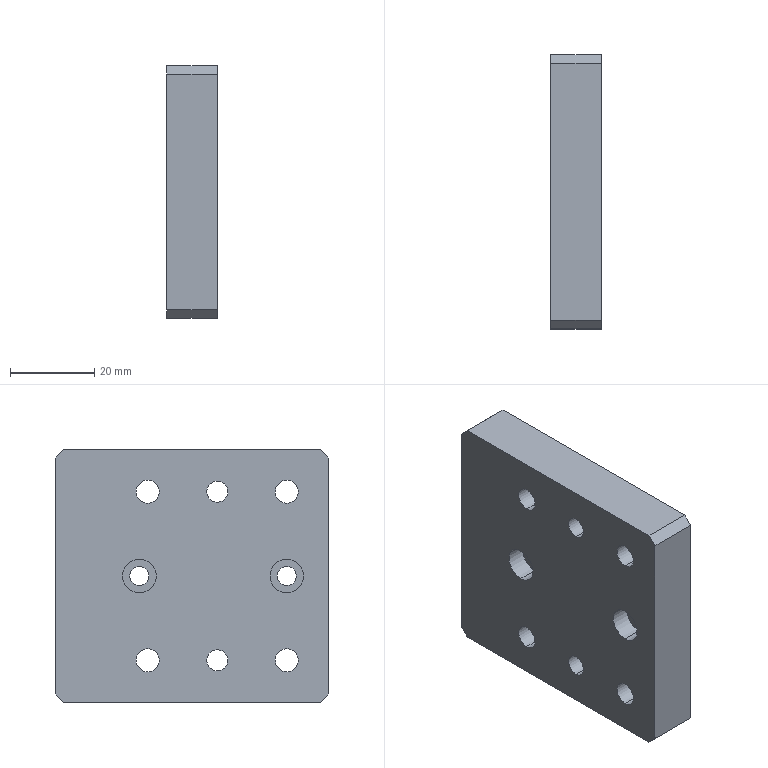Part | SolidWorks | features HoleWzd 3, Chamfer 1, Extrusion 1 | 1 solid | 44 faces | box 12 x 65 x 60 mm | volume 43146 mm3 | cylinder 28 | plane 16 | commonest cylinder face diameters 5.5 x8 10 x8 4.5 x4 5 x4 8 x4
STEP:
#1=CARTESIAN_POINT('',(0.,-6.,-17.5));
#2=VERTEX_POINT('',#1);
#3=CARTESIAN_POINT('',(0.,-6.,-22.5));
#4=VERTEX_POINT('',#3);
#5=CARTESIAN_POINT('',(0.,-6.,-20.));
#6=DIRECTION('',(1.,0.,0.));
#7=DIRECTION('',(0.,0.,-1.));
#8=AXIS2_PLACEMENT_3D('',#5,#6,#7);
#9=CIRCLE('',#8,2.5);
#10=EDGE_CURVE('',#2,#4,#9,.T.);
#11=ORIENTED_EDGE('',*,*,#10,.F.);
#12=CARTESIAN_POINT('',(12.,-6.,-17.5));
#13=VERTEX_POINT('',#12);
#14=CARTESIAN_POINT('',(12.,-6.,-17.5));
#15=DIRECTION('',(1.,0.,0.));
#16=VECTOR('',#15,1000.);
#17=LINE('',#14,#16);
#18=EDGE_CURVE('',#2,#13,#17,.T.);
#19=ORIENTED_EDGE('',*,*,#18,.T.);
#20=CARTESIAN_POINT('',(12.,-6.,-22.5));
#21=VERTEX_POINT('',#20);
#22=CARTESIAN_POINT('',(12.,-6.,-20.));
#23=DIRECTION('',(1.,0.,0.));
#24=DIRECTION('',(0.,0.,-1.));
#25=AXIS2_PLACEMENT_3D('',#22,#23,#24);
#26=CIRCLE('',#25,2.5);
#27=EDGE_CURVE('',#13,#21,#26,.T.);
#28=ORIENTED_EDGE('',*,*,#27,.T.);
#29=CARTESIAN_POINT('',(12.,-6.,-22.5));
#30=DIRECTION('',(1.,0.,0.));
#31=VECTOR('',#30,1000.);
#32=LINE('',#29,#31);
#33=EDGE_CURVE('',#4,#21,#32,.T.);
#34=ORIENTED_EDGE('',*,*,#33,.F.);
#35=EDGE_LOOP('',(#11,#19,#28,#34));
#36=FACE_OUTER_BOUND('',#35,.T.);
#37=CARTESIAN_POINT('',(12.,-6.,-20.));
#38=DIRECTION('',(1.,0.,0.));
#39=DIRECTION('',(0.,0.,-1.));
#40=AXIS2_PLACEMENT_3D('',#37,#38,#39);
#41=CYLINDRICAL_SURFACE('',#40,2.5);
#42=ADVANCED_FACE('',(#36),#41,.F.);
#43=CARTESIAN_POINT('',(0.,-6.,22.5));
#44=VERTEX_POINT('',#43);
#45=CARTESIAN_POINT('',(0.,-6.,17.5));
#46=VERTEX_POINT('',#45);
#47=CARTESIAN_POINT('',(0.,-6.,20.));
#48=DIRECTION('',(1.,0.,0.));
#49=DIRECTION('',(0.,0.,-1.));
#50=AXIS2_PLACEMENT_3D('',#47,#48,#49);
#51=CIRCLE('',#50,2.5);
#52=EDGE_CURVE('',#44,#46,#51,.T.);
#53=ORIENTED_EDGE('',*,*,#52,.F.);
#54=CARTESIAN_POINT('',(12.,-6.,22.5));
#55=VERTEX_POINT('',#54);
#56=CARTESIAN_POINT('',(12.,-6.,22.5));
#57=DIRECTION('',(1.,0.,0.));
#58=VECTOR('',#57,1000.);
#59=LINE('',#56,#58);
#60=EDGE_CURVE('',#44,#55,#59,.T.);
#61=ORIENTED_EDGE('',*,*,#60,.T.);
#62=CARTESIAN_POINT('',(12.,-6.,17.5));
#63=VERTEX_POINT('',#62);
#64=CARTESIAN_POINT('',(12.,-6.,20.));
#65=DIRECTION('',(1.,0.,0.));
#66=DIRECTION('',(0.,0.,-1.));
#67=AXIS2_PLACEMENT_3D('',#64,#65,#66);
#68=CIRCLE('',#67,2.5);
#69=EDGE_CURVE('',#55,#63,#68,.T.);
#70=ORIENTED_EDGE('',*,*,#69,.T.);
#71=CARTESIAN_POINT('',(12.,-6.,17.5));
#72=DIRECTION('',(1.,0.,0.));
#73=VECTOR('',#72,1000.);
#74=LINE('',#71,#73);
#75=EDGE_CURVE('',#46,#63,#74,.T.);
#76=ORIENTED_EDGE('',*,*,#75,.F.);
#77=EDGE_LOOP('',(#53,#61,#70,#76));
#78=FACE_OUTER_BOUND('',#77,.T.);
#79=CARTESIAN_POINT('',(12.,-6.,20.));
#80=DIRECTION('',(1.,0.,0.));
#81=DIRECTION('',(0.,0.,-1.));
#82=AXIS2_PLACEMENT_3D('',#79,#80,#81);
#83=CYLINDRICAL_SURFACE('',#82,2.5);
#84=ADVANCED_FACE('',(#78),#83,.F.);
#85=CARTESIAN_POINT('',(6.3,10.5,25.));
#86=VERTEX_POINT('',#85);
#87=CARTESIAN_POINT('',(6.3,10.5,15.));
#88=VERTEX_POINT('',#87);
#89=CARTESIAN_POINT('',(6.3,10.5,20.));
#90=DIRECTION('',(1.,0.,0.));
#91=DIRECTION('',(0.,0.,-1.));
#92=AXIS2_PLACEMENT_3D('',#89,#90,#91);
#93=CIRCLE('',#92,5.);
#94=EDGE_CURVE('',#86,#88,#93,.T.);
#95=ORIENTED_EDGE('',*,*,#94,.F.);
#96=CARTESIAN_POINT('',(12.,10.5,25.));
#97=VERTEX_POINT('',#96);
#98=CARTESIAN_POINT('',(12.,10.5,25.));
#99=DIRECTION('',(1.,0.,0.));
#100=VECTOR('',#99,1000.);
#101=LINE('',#98,#100);
#102=EDGE_CURVE('',#86,#97,#101,.T.);
#103=ORIENTED_EDGE('',*,*,#102,.T.);
#104=CARTESIAN_POINT('',(12.,10.5,15.));
#105=VERTEX_POINT('',#104);
#106=CARTESIAN_POINT('',(12.,10.5,20.));
#107=DIRECTION('',(1.,0.,0.));
#108=DIRECTION('',(0.,0.,-1.));
#109=AXIS2_PLACEMENT_3D('',#106,#107,#108);
#110=CIRCLE('',#109,5.);
#111=EDGE_CURVE('',#97,#105,#110,.T.);
#112=ORIENTED_EDGE('',*,*,#111,.T.);
#113=CARTESIAN_POINT('',(12.,10.5,15.));
#114=DIRECTION('',(1.,0.,0.));
#115=VECTOR('',#114,1000.);
#116=LINE('',#113,#115);
#117=EDGE_CURVE('',#88,#105,#116,.T.);
#118=ORIENTED_EDGE('',*,*,#117,.F.);
#119=EDGE_LOOP('',(#95,#103,#112,#118));
#120=FACE_OUTER_BOUND('',#119,.T.);
#121=CARTESIAN_POINT('',(12.,10.5,20.));
#122=DIRECTION('',(1.,0.,0.));
#123=DIRECTION('',(0.,0.,-1.));
#124=AXIS2_PLACEMENT_3D('',#121,#122,#123);
#125=CYLINDRICAL_SURFACE('',#124,5.);
#126=ADVANCED_FACE('',(#120),#125,.F.);
#127=CARTESIAN_POINT('',(0.,10.5,22.75));
#128=VERTEX_POINT('',#127);
#129=CARTESIAN_POINT('',(0.,10.5,17.25));
#130=VERTEX_POINT('',#129);
#131=CARTESIAN_POINT('',(0.,10.5,20.));
#132=DIRECTION('',(1.,0.,0.));
#133=DIRECTION('',(0.,0.,-1.));
#134=AXIS2_PLACEMENT_3D('',#131,#132,#133);
#135=CIRCLE('',#134,2.75);
#136=EDGE_CURVE('',#128,#130,#135,.T.);
#137=ORIENTED_EDGE('',*,*,#136,.F.);
#138=CARTESIAN_POINT('',(6.3,10.5,22.75));
#139=VERTEX_POINT('',#138);
#140=CARTESIAN_POINT('',(12.,10.5,22.75));
#141=DIRECTION('',(1.,0.,0.));
#142=VECTOR('',#141,1000.);
#143=LINE('',#140,#142);
#144=EDGE_CURVE('',#128,#139,#143,.T.);
#145=ORIENTED_EDGE('',*,*,#144,.T.);
#146=CARTESIAN_POINT('',(6.3,10.5,17.25));
#147=VERTEX_POINT('',#146);
#148=CARTESIAN_POINT('',(6.3,10.5,20.));
#149=DIRECTION('',(1.,0.,0.));
#150=DIRECTION('',(0.,0.,-1.));
#151=AXIS2_PLACEMENT_3D('',#148,#149,#150);
#152=CIRCLE('',#151,2.75);
#153=EDGE_CURVE('',#139,#147,#152,.T.);
#154=ORIENTED_EDGE('',*,*,#153,.T.);
#155=CARTESIAN_POINT('',(12.,10.5,17.25));
#156=DIRECTION('',(1.,0.,0.));
#157=VECTOR('',#156,1000.);
#158=LINE('',#155,#157);
#159=EDGE_CURVE('',#130,#147,#158,.T.);
#160=ORIENTED_EDGE('',*,*,#159,.F.);
#161=EDGE_LOOP('',(#137,#145,#154,#160));
#162=FACE_OUTER_BOUND('',#161,.T.);
#163=CARTESIAN_POINT('',(12.,10.5,20.));
#164=DIRECTION('',(1.,0.,0.));
#165=DIRECTION('',(0.,0.,-1.));
#166=AXIS2_PLACEMENT_3D('',#163,#164,#165);
#167=CYLINDRICAL_SURFACE('',#166,2.75);
#168=ADVANCED_FACE('',(#162),#167,.F.);
#169=CARTESIAN_POINT('',(6.3,-22.5,25.));
#170=VERTEX_POINT('',#169);
#171=CARTESIAN_POINT('',(6.3,-22.5,15.));
#172=VERTEX_POINT('',#171);
#173=CARTESIAN_POINT('',(6.3,-22.5,20.));
#174=DIRECTION('',(1.,0.,0.));
#175=DIRECTION('',(0.,0.,-1.));
#176=AXIS2_PLACEMENT_3D('',#173,#174,#175);
#177=CIRCLE('',#176,5.);
#178=EDGE_CURVE('',#170,#172,#177,.T.);
#179=ORIENTED_EDGE('',*,*,#178,.F.);
#180=CARTESIAN_POINT('',(12.,-22.5,25.));
#181=VERTEX_POINT('',#180);
#182=CARTESIAN_POINT('',(12.,-22.5,25.));
#183=DIRECTION('',(1.,0.,0.));
#184=VECTOR('',#183,1000.);
#185=LINE('',#182,#184);
#186=EDGE_CURVE('',#170,#181,#185,.T.);
#187=ORIENTED_EDGE('',*,*,#186,.T.);
#188=CARTESIAN_POINT('',(12.,-22.5,15.));
#189=VERTEX_POINT('',#188);
#190=CARTESIAN_POINT('',(12.,-22.5,20.));
#191=DIRECTION('',(1.,0.,0.));
#192=DIRECTION('',(0.,0.,-1.));
#193=AXIS2_PLACEMENT_3D('',#190,#191,#192);
#194=CIRCLE('',#193,5.);
#195=EDGE_CURVE('',#181,#189,#194,.T.);
#196=ORIENTED_EDGE('',*,*,#195,.T.);
#197=CARTESIAN_POINT('',(12.,-22.5,15.));
#198=DIRECTION('',(1.,0.,0.));
#199=VECTOR('',#198,1000.);
#200=LINE('',#197,#199);
#201=EDGE_CURVE('',#172,#189,#200,.T.);
#202=ORIENTED_EDGE('',*,*,#201,.F.);
#203=EDGE_LOOP('',(#179,#187,#196,#202));
#204=FACE_OUTER_BOUND('',#203,.T.);
#205=CARTESIAN_POINT('',(12.,-22.5,20.));
#206=DIRECTION('',(1.,0.,0.));
#207=DIRECTION('',(0.,0.,-1.));
#208=AXIS2_PLACEMENT_3D('',#205,#206,#207);
#209=CYLINDRICAL_SURFACE('',#208,5.);
#210=ADVANCED_FACE('',(#204),#209,.F.);
#211=CARTESIAN_POINT('',(0.,-22.5,22.75));
#212=VERTEX_POINT('',#211);
#213=CARTESIAN_POINT('',(0.,-22.5,17.25));
#214=VERTEX_POINT('',#213);
#215=CARTESIAN_POINT('',(0.,-22.5,20.));
#216=DIRECTION('',(1.,0.,0.));
#217=DIRECTION('',(0.,0.,-1.));
#218=AXIS2_PLACEMENT_3D('',#215,#216,#217);
#219=CIRCLE('',#218,2.75);
#220=EDGE_CURVE('',#212,#214,#219,.T.);
#221=ORIENTED_EDGE('',*,*,#220,.F.);
#222=CARTESIAN_POINT('',(6.3,-22.5,22.75));
#223=VERTEX_POINT('',#222);
#224=CARTESIAN_POINT('',(12.,-22.5,22.75));
#225=DIRECTION('',(1.,0.,0.));
#226=VECTOR('',#225,1000.);
#227=LINE('',#224,#226);
#228=EDGE_CURVE('',#212,#223,#227,.T.);
#229=ORIENTED_EDGE('',*,*,#228,.T.);
#230=CARTESIAN_POINT('',(6.3,-22.5,17.25));
#231=VERTEX_POINT('',#230);
#232=CARTESIAN_POINT('',(6.3,-22.5,20.));
#233=DIRECTION('',(1.,0.,0.));
#234=DIRECTION('',(0.,0.,-1.));
#235=AXIS2_PLACEMENT_3D('',#232,#233,#234);
#236=CIRCLE('',#235,2.75);
#237=EDGE_CURVE('',#223,#231,#236,.T.);
#238=ORIENTED_EDGE('',*,*,#237,.T.);
#239=CARTESIAN_POINT('',(12.,-22.5,17.25));
#240=DIRECTION('',(1.,0.,0.));
#241=VECTOR('',#240,1000.);
#242=LINE('',#239,#241);
#243=EDGE_CURVE('',#214,#231,#242,.T.);
#244=ORIENTED_EDGE('',*,*,#243,.F.);
#245=EDGE_LOOP('',(#221,#229,#238,#244));
#246=FACE_OUTER_BOUND('',#245,.T.);
#247=CARTESIAN_POINT('',(12.,-22.5,20.));
#248=DIRECTION('',(1.,0.,0.));
#249=DIRECTION('',(0.,0.,-1.));
#250=AXIS2_PLACEMENT_3D('',#247,#248,#249);
#251=CYLINDRICAL_SURFACE('',#250,2.75);
#252=ADVANCED_FACE('',(#246),#251,.F.);
#253=CARTESIAN_POINT('',(6.3,-22.5,-15.));
#254=VERTEX_POINT('',#253);
#255=CARTESIAN_POINT('',(6.3,-22.5,-25.));
#256=VERTEX_POINT('',#255);
#257=CARTESIAN_POINT('',(6.3,-22.5,-20.));
#258=DIRECTION('',(1.,0.,0.));
#259=DIRECTION('',(0.,0.,-1.));
#260=AXIS2_PLACEMENT_3D('',#257,#258,#259);
#261=CIRCLE('',#260,5.);
#262=EDGE_CURVE('',#254,#256,#261,.T.);
#263=ORIENTED_EDGE('',*,*,#262,.F.);
#264=CARTESIAN_POINT('',(12.,-22.5,-15.));
#265=VERTEX_POINT('',#264);
#266=CARTESIAN_POINT('',(12.,-22.5,-15.));
#267=DIRECTION('',(1.,0.,0.));
#268=VECTOR('',#267,1000.);
#269=LINE('',#266,#268);
#270=EDGE_CURVE('',#254,#265,#269,.T.);
#271=ORIENTED_EDGE('',*,*,#270,.T.);
#272=CARTESIAN_POINT('',(12.,-22.5,-25.));
#273=VERTEX_POINT('',#272);
#274=CARTESIAN_POINT('',(12.,-22.5,-20.));
#275=DIRECTION('',(1.,0.,0.));
#276=DIRECTION('',(0.,0.,-1.));
#277=AXIS2_PLACEMENT_3D('',#274,#275,#276);
#278=CIRCLE('',#277,5.);
#279=EDGE_CURVE('',#265,#273,#278,.T.);
#280=ORIENTED_EDGE('',*,*,#279,.T.);
#281=CARTESIAN_POINT('',(12.,-22.5,-25.));
#282=DIRECTION('',(1.,0.,0.));
#283=VECTOR('',#282,1000.);
#284=LINE('',#281,#283);
#285=EDGE_CURVE('',#256,#273,#284,.T.);
#286=ORIENTED_EDGE('',*,*,#285,.F.);
#287=EDGE_LOOP('',(#263,#271,#280,#286));
#288=FACE_OUTER_BOUND('',#287,.T.);
#289=CARTESIAN_POINT('',(12.,-22.5,-20.));
#290=DIRECTION('',(1.,0.,0.));
#291=DIRECTION('',(0.,0.,-1.));
#292=AXIS2_PLACEMENT_3D('',#289,#290,#291);
#293=CYLINDRICAL_SURFACE('',#292,5.);
#294=ADVANCED_FACE('',(#288),#293,.F.);
#295=CARTESIAN_POINT('',(0.,-22.5,-17.25));
#296=VERTEX_POINT('',#295);
#297=CARTESIAN_POINT('',(0.,-22.5,-22.75));
#298=VERTEX_POINT('',#297);
#299=CARTESIAN_POINT('',(0.,-22.5,-20.));
#300=DIRECTION('',(1.,0.,0.));
#301=DIRECTION('',(0.,0.,-1.));
#302=AXIS2_PLACEMENT_3D('',#299,#300,#301);
#303=CIRCLE('',#302,2.75);
#304=EDGE_CURVE('',#296,#298,#303,.T.);
#305=ORIENTED_EDGE('',*,*,#304,.F.);
#306=CARTESIAN_POINT('',(6.3,-22.5,-17.25));
#307=VERTEX_POINT('',#306);
#308=CARTESIAN_POINT('',(12.,-22.5,-17.25));
#309=DIRECTION('',(1.,0.,0.));
#310=VECTOR('',#309,1000.);
#311=LINE('',#308,#310);
#312=EDGE_CURVE('',#296,#307,#311,.T.);
#313=ORIENTED_EDGE('',*,*,#312,.T.);
#314=CARTESIAN_POINT('',(6.3,-22.5,-22.75));
#315=VERTEX_POINT('',#314);
#316=CARTESIAN_POINT('',(6.3,-22.5,-20.));
#317=DIRECTION('',(1.,0.,0.));
#318=DIRECTION('',(0.,0.,-1.));
#319=AXIS2_PLACEMENT_3D('',#316,#317,#318);
#320=CIRCLE('',#319,2.75);
#321=EDGE_CURVE('',#307,#315,#320,.T.);
#322=ORIENTED_EDGE('',*,*,#321,.T.);
#323=CARTESIAN_POINT('',(12.,-22.5,-22.75));
#324=DIRECTION('',(1.,0.,0.));
#325=VECTOR('',#324,1000.);
#326=LINE('',#323,#325);
#327=EDGE_CURVE('',#298,#315,#326,.T.);
#328=ORIENTED_EDGE('',*,*,#327,.F.);
#329=EDGE_LOOP('',(#305,#313,#322,#328));
#330=FACE_OUTER_BOUND('',#329,.T.);
#331=CARTESIAN_POINT('',(12.,-22.5,-20.));
#332=DIRECTION('',(1.,0.,0.));
#333=DIRECTION('',(0.,0.,-1.));
#334=AXIS2_PLACEMENT_3D('',#331,#332,#333);
#335=CYLINDRICAL_SURFACE('',#334,2.75);
#336=ADVANCED_FACE('',(#330),#335,.F.);
#337=CARTESIAN_POINT('',(6.3,10.5,-15.));
#338=VERTEX_POINT('',#337);
#339=CARTESIAN_POINT('',(6.3,10.5,-25.));
#340=VERTEX_POINT('',#339);
#341=CARTESIAN_POINT('',(6.3,10.5,-20.));
#342=DIRECTION('',(1.,0.,0.));
#343=DIRECTION('',(0.,0.,-1.));
#344=AXIS2_PLACEMENT_3D('',#341,#342,#343);
#345=CIRCLE('',#344,5.);
#346=EDGE_CURVE('',#338,#340,#345,.T.);
#347=ORIENTED_EDGE('',*,*,#346,.F.);
#348=CARTESIAN_POINT('',(12.,10.5,-15.));
#349=VERTEX_POINT('',#348);
#350=CARTESIAN_POINT('',(12.,10.5,-15.));
#351=DIRECTION('',(1.,0.,0.));
#352=VECTOR('',#351,1000.);
#353=LINE('',#350,#352);
#354=EDGE_CURVE('',#338,#349,#353,.T.);
#355=ORIENTED_EDGE('',*,*,#354,.T.);
#356=CARTESIAN_POINT('',(12.,10.5,-25.));
#357=VERTEX_POINT('',#356);
#358=CARTESIAN_POINT('',(12.,10.5,-20.));
#359=DIRECTION('',(1.,0.,0.));
#360=DIRECTION('',(0.,0.,-1.));
#361=AXIS2_PLACEMENT_3D('',#358,#359,#360);
#362=CIRCLE('',#361,5.);
#363=EDGE_CURVE('',#349,#357,#362,.T.);
#364=ORIENTED_EDGE('',*,*,#363,.T.);
#365=CARTESIAN_POINT('',(12.,10.5,-25.));
#366=DIRECTION('',(1.,0.,0.));
#367=VECTOR('',#366,1000.);
#368=LINE('',#365,#367);
#369=EDGE_CURVE('',#340,#357,#368,.T.);
#370=ORIENTED_EDGE('',*,*,#369,.F.);
#371=EDGE_LOOP('',(#347,#355,#364,#370));
#372=FACE_OUTER_BOUND('',#371,.T.);
#373=CARTESIAN_POINT('',(12.,10.5,-20.));
#374=DIRECTION('',(1.,0.,0.));
#375=DIRECTION('',(0.,0.,-1.));
#376=AXIS2_PLACEMENT_3D('',#373,#374,#375);
#377=CYLINDRICAL_SURFACE('',#376,5.);
#378=ADVANCED_FACE('',(#372),#377,.F.);
#379=CARTESIAN_POINT('',(0.,10.5,-17.25));
#380=VERTEX_POINT('',#379);
#381=CARTESIAN_POINT('',(0.,10.5,-22.75));
#382=VERTEX_POINT('',#381);
#383=CARTESIAN_POINT('',(0.,10.5,-20.));
#384=DIRECTION('',(1.,0.,0.));
#385=DIRECTION('',(0.,0.,-1.));
#386=AXIS2_PLACEMENT_3D('',#383,#384,#385);
#387=CIRCLE('',#386,2.75);
#388=EDGE_CURVE('',#380,#382,#387,.T.);
#389=ORIENTED_EDGE('',*,*,#388,.F.);
#390=CARTESIAN_POINT('',(6.3,10.5,-17.25));
#391=VERTEX_POINT('',#390);
#392=CARTESIAN_POINT('',(12.,10.5,-17.25));
#393=DIRECTION('',(1.,0.,0.));
#394=VECTOR('',#393,1000.);
#395=LINE('',#392,#394);
#396=EDGE_CURVE('',#380,#391,#395,.T.);
#397=ORIENTED_EDGE('',*,*,#396,.T.);
#398=CARTESIAN_POINT('',(6.3,10.5,-22.75));
#399=VERTEX_POINT('',#398);
#400=CARTESIAN_POINT('',(6.3,10.5,-20.));
#401=DIRECTION('',(1.,0.,0.));
#402=DIRECTION('',(0.,0.,-1.));
#403=AXIS2_PLACEMENT_3D('',#400,#401,#402);
#404=CIRCLE('',#403,2.75);
#405=EDGE_CURVE('',#391,#399,#404,.T.);
#406=ORIENTED_EDGE('',*,*,#405,.T.);
#407=CARTESIAN_POINT('',(12.,10.5,-22.75));
#408=DIRECTION('',(1.,0.,0.));
#409=VECTOR('',#408,1000.);
#410=LINE('',#407,#409);
#411=EDGE_CURVE('',#382,#399,#410,.T.);
#412=ORIENTED_EDGE('',*,*,#411,.F.);
#413=EDGE_LOOP('',(#389,#397,#406,#412));
#414=FACE_OUTER_BOUND('',#413,.T.);
#415=CARTESIAN_POINT('',(12.,10.5,-20.));
#416=DIRECTION('',(1.,0.,0.));
#417=DIRECTION('',(0.,0.,-1.));
#418=AXIS2_PLACEMENT_3D('',#415,#416,#417);
#419=CYLINDRICAL_SURFACE('',#418,2.75);
#420=ADVANCED_FACE('',(#414),#419,.F.);
#421=CARTESIAN_POINT('',(4.6,12.5,-4.));
#422=VERTEX_POINT('',#421);
#423=CARTESIAN_POINT('',(4.6,12.5,4.));
#424=VERTEX_POINT('',#423);
#425=CARTESIAN_POINT('',(4.6,12.5,0.));
#426=DIRECTION('',(-1.,0.,0.));
#427=DIRECTION('',(0.,0.,1.));
#428=AXIS2_PLACEMENT_3D('',#425,#426,#427);
#429=CIRCLE('',#428,4.);
#430=EDGE_CURVE('',#422,#424,#429,.T.);
#431=ORIENTED_EDGE('',*,*,#430,.F.);
#432=CARTESIAN_POINT('',(0.,12.5,-4.));
#433=VERTEX_POINT('',#432);
#434=CARTESIAN_POINT('',(0.,12.5,-4.));
#435=DIRECTION('',(-1.,0.,0.));
#436=VECTOR('',#435,1000.);
#437=LINE('',#434,#436);
#438=EDGE_CURVE('',#422,#433,#437,.T.);
#439=ORIENTED_EDGE('',*,*,#438,.T.);
#440=CARTESIAN_POINT('',(0.,12.5,4.));
#441=VERTEX_POINT('',#440);
#442=CARTESIAN_POINT('',(0.,12.5,0.));
#443=DIRECTION('',(-1.,0.,0.));
#444=DIRECTION('',(0.,0.,1.));
#445=AXIS2_PLACEMENT_3D('',#442,#443,#444);
#446=CIRCLE('',#445,4.);
#447=EDGE_CURVE('',#433,#441,#446,.T.);
#448=ORIENTED_EDGE('',*,*,#447,.T.);
#449=CARTESIAN_POINT('',(0.,12.5,4.));
#450=DIRECTION('',(-1.,0.,0.));
#451=VECTOR('',#450,1000.);
#452=LINE('',#449,#451);
#453=EDGE_CURVE('',#424,#441,#452,.T.);
#454=ORIENTED_EDGE('',*,*,#453,.F.);
#455=EDGE_LOOP('',(#431,#439,#448,#454));
#456=FACE_OUTER_BOUND('',#455,.T.);
#457=CARTESIAN_POINT('',(0.,12.5,0.));
#458=DIRECTION('',(-1.,0.,0.));
#459=DIRECTION('',(0.,0.,1.));
#460=AXIS2_PLACEMENT_3D('',#457,#458,#459);
#461=CYLINDRICAL_SURFACE('',#460,4.);
#462=ADVANCED_FACE('',(#456),#461,.F.);
#463=CARTESIAN_POINT('',(12.,12.5,-2.25));
#464=VERTEX_POINT('',#463);
#465=CARTESIAN_POINT('',(12.,12.5,2.25));
#466=VERTEX_POINT('',#465);
#467=CARTESIAN_POINT('',(12.,12.5,0.));
#468=DIRECTION('',(-1.,0.,0.));
#469=DIRECTION('',(0.,0.,1.));
#470=AXIS2_PLACEMENT_3D('',#467,#468,#469);
#471=CIRCLE('',#470,2.25);
#472=EDGE_CURVE('',#464,#466,#471,.T.);
#473=ORIENTED_EDGE('',*,*,#472,.F.);
#474=CARTESIAN_POINT('',(4.6,12.5,-2.25));
#475=VERTEX_POINT('',#474);
#476=CARTESIAN_POINT('',(0.,12.5,-2.25));
#477=DIRECTION('',(-1.,0.,0.));
#478=VECTOR('',#477,1000.);
#479=LINE('',#476,#478);
#480=EDGE_CURVE('',#464,#475,#479,.T.);
#481=ORIENTED_EDGE('',*,*,#480,.T.);
#482=CARTESIAN_POINT('',(4.6,12.5,2.25));
#483=VERTEX_POINT('',#482);
#484=CARTESIAN_POINT('',(4.6,12.5,0.));
#485=DIRECTION('',(-1.,0.,0.));
#486=DIRECTION('',(0.,0.,1.));
#487=AXIS2_PLACEMENT_3D('',#484,#485,#486);
#488=CIRCLE('',#487,2.25);
#489=EDGE_CURVE('',#475,#483,#488,.T.);
#490=ORIENTED_EDGE('',*,*,#489,.T.);
#491=CARTESIAN_POINT('',(0.,12.5,2.25));
#492=DIRECTION('',(-1.,0.,0.));
#493=VECTOR('',#492,1000.);
#494=LINE('',#491,#493);
#495=EDGE_CURVE('',#466,#483,#494,.T.);
#496=ORIENTED_EDGE('',*,*,#495,.F.);
#497=EDGE_LOOP('',(#473,#481,#490,#496));
#498=FACE_OUTER_BOUND('',#497,.T.);
#499=CARTESIAN_POINT('',(0.,12.5,0.));
#500=DIRECTION('',(-1.,0.,0.));
#501=DIRECTION('',(0.,0.,1.));
#502=AXIS2_PLACEMENT_3D('',#499,#500,#501);
#503=CYLINDRICAL_SURFACE('',#502,2.25);
#504=ADVANCED_FACE('',(#498),#503,.F.);
#505=CARTESIAN_POINT('',(4.6,-22.5,-4.));
#506=VERTEX_POINT('',#505);
#507=CARTESIAN_POINT('',(4.6,-22.5,4.));
#508=VERTEX_POINT('',#507);
#509=CARTESIAN_POINT('',(4.6,-22.5,0.));
#510=DIRECTION('',(-1.,0.,0.));
#511=DIRECTION('',(0.,0.,1.));
#512=AXIS2_PLACEMENT_3D('',#509,#510,#511);
#513=CIRCLE('',#512,4.);
#514=EDGE_CURVE('',#506,#508,#513,.T.);
#515=ORIENTED_EDGE('',*,*,#514,.F.);
#516=CARTESIAN_POINT('',(0.,-22.5,-4.));
#517=VERTEX_POINT('',#516);
#518=CARTESIAN_POINT('',(0.,-22.5,-4.));
#519=DIRECTION('',(-1.,0.,0.));
#520=VECTOR('',#519,1000.);
#521=LINE('',#518,#520);
#522=EDGE_CURVE('',#506,#517,#521,.T.);
#523=ORIENTED_EDGE('',*,*,#522,.T.);
#524=CARTESIAN_POINT('',(0.,-22.5,4.));
#525=VERTEX_POINT('',#524);
#526=CARTESIAN_POINT('',(0.,-22.5,0.));
#527=DIRECTION('',(-1.,0.,0.));
#528=DIRECTION('',(0.,0.,1.));
#529=AXIS2_PLACEMENT_3D('',#526,#527,#528);
#530=CIRCLE('',#529,4.);
#531=EDGE_CURVE('',#517,#525,#530,.T.);
#532=ORIENTED_EDGE('',*,*,#531,.T.);
#533=CARTESIAN_POINT('',(0.,-22.5,4.));
#534=DIRECTION('',(-1.,0.,0.));
#535=VECTOR('',#534,1000.);
#536=LINE('',#533,#535);
#537=EDGE_CURVE('',#508,#525,#536,.T.);
#538=ORIENTED_EDGE('',*,*,#537,.F.);
#539=EDGE_LOOP('',(#515,#523,#532,#538));
#540=FACE_OUTER_BOUND('',#539,.T.);
#541=CARTESIAN_POINT('',(0.,-22.5,0.));
#542=DIRECTION('',(-1.,0.,0.));
#543=DIRECTION('',(0.,0.,1.));
#544=AXIS2_PLACEMENT_3D('',#541,#542,#543);
#545=CYLINDRICAL_SURFACE('',#544,4.);
#546=ADVANCED_FACE('',(#540),#545,.F.);
#547=CARTESIAN_POINT('',(12.,-22.5,-2.25));
#548=VERTEX_POINT('',#547);
#549=CARTESIAN_POINT('',(12.,-22.5,2.25));
#550=VERTEX_POINT('',#549);
#551=CARTESIAN_POINT('',(12.,-22.5,0.));
#552=DIRECTION('',(-1.,0.,0.));
#553=DIRECTION('',(0.,0.,1.));
#554=AXIS2_PLACEMENT_3D('',#551,#552,#553);
#555=CIRCLE('',#554,2.25);
#556=EDGE_CURVE('',#548,#550,#555,.T.);
#557=ORIENTED_EDGE('',*,*,#556,.F.);
#558=CARTESIAN_POINT('',(4.6,-22.5,-2.25));
#559=VERTEX_POINT('',#558);
#560=CARTESIAN_POINT('',(0.,-22.5,-2.25));
#561=DIRECTION('',(-1.,0.,0.));
#562=VECTOR('',#561,1000.);
#563=LINE('',#560,#562);
#564=EDGE_CURVE('',#548,#559,#563,.T.);
#565=ORIENTED_EDGE('',*,*,#564,.T.);
#566=CARTESIAN_POINT('',(4.6,-22.5,2.25));
#567=VERTEX_POINT('',#566);
#568=CARTESIAN_POINT('',(4.6,-22.5,0.));
#569=DIRECTION('',(-1.,0.,0.));
#570=DIRECTION('',(0.,0.,1.));
#571=AXIS2_PLACEMENT_3D('',#568,#569,#570);
#572=CIRCLE('',#571,2.25);
#573=EDGE_CURVE('',#559,#567,#572,.T.);
#574=ORIENTED_EDGE('',*,*,#573,.T.);
#575=CARTESIAN_POINT('',(0.,-22.5,2.25));
#576=DIRECTION('',(-1.,0.,0.));
#577=VECTOR('',#576,1000.);
#578=LINE('',#575,#577);
#579=EDGE_CURVE('',#550,#567,#578,.T.);
#580=ORIENTED_EDGE('',*,*,#579,.F.);
#581=EDGE_LOOP('',(#557,#565,#574,#580));
#582=FACE_OUTER_BOUND('',#581,.T.);
#583=CARTESIAN_POINT('',(0.,-22.5,0.));
#584=DIRECTION('',(-1.,0.,0.));
#585=DIRECTION('',(0.,0.,1.));
#586=AXIS2_PLACEMENT_3D('',#583,#584,#585);
#587=CYLINDRICAL_SURFACE('',#586,2.25);
#588=ADVANCED_FACE('',(#582),#587,.F.);
#589=CARTESIAN_POINT('',(12.,-30.5,-30.));
#590=VERTEX_POINT('',#589);
#591=CARTESIAN_POINT('',(12.,30.5,-30.));
#592=VERTEX_POINT('',#591);
#593=CARTESIAN_POINT('',(12.,-32.5,-30.));
#594=DIRECTION('',(0.,1.,0.));
#595=VECTOR('',#594,1000.);
#596=LINE('',#593,#595);
#597=EDGE_CURVE('',#590,#592,#596,.T.);
#598=ORIENTED_EDGE('',*,*,#597,.F.);
#599=CARTESIAN_POINT('',(0.,-30.5,-30.));
#600=VERTEX_POINT('',#599);
#601=CARTESIAN_POINT('',(12.,-30.5,-30.));
#602=DIRECTION('',(-1.,0.,0.));
#603=VECTOR('',#602,1000.);
#604=LINE('',#601,#603);
#605=EDGE_CURVE('',#590,#600,#604,.T.);
#606=ORIENTED_EDGE('',*,*,#605,.T.);
#607=CARTESIAN_POINT('',(0.,30.5,-30.));
#608=VERTEX_POINT('',#607);
#609=CARTESIAN_POINT('',(0.,-32.5,-30.));
#610=DIRECTION('',(0.,1.,0.));
#611=VECTOR('',#610,1000.);
#612=LINE('',#609,#611);
#613=EDGE_CURVE('',#600,#608,#612,.T.);
#614=ORIENTED_EDGE('',*,*,#613,.T.);
#615=CARTESIAN_POINT('',(12.,30.5,-30.));
#616=DIRECTION('',(1.,0.,0.));
#617=VECTOR('',#616,1000.);
#618=LINE('',#615,#617);
#619=EDGE_CURVE('',#608,#592,#618,.T.);
#620=ORIENTED_EDGE('',*,*,#619,.T.);
#621=EDGE_LOOP('',(#598,#606,#614,#620));
#622=FACE_OUTER_BOUND('',#621,.T.);
#623=CARTESIAN_POINT('',(12.,-32.5,-30.));
#624=DIRECTION('',(0.,0.,1.));
#625=DIRECTION('',(1.,0.,0.));
#626=AXIS2_PLACEMENT_3D('',#623,#624,#625);
#627=PLANE('',#626);
#628=ADVANCED_FACE('',(#622),#627,.F.);
#629=CARTESIAN_POINT('',(0.,32.5,-28.));
#630=VERTEX_POINT('',#629);
#631=CARTESIAN_POINT('',(0.,32.5,28.));
#632=VERTEX_POINT('',#631);
#633=CARTESIAN_POINT('',(0.,32.5,30.));
#634=DIRECTION('',(0.,0.,1.));
#635=VECTOR('',#634,1000.);
#636=LINE('',#633,#635);
#637=EDGE_CURVE('',#630,#632,#636,.T.);
#638=ORIENTED_EDGE('',*,*,#637,.T.);
#639=CARTESIAN_POINT('',(12.,32.5,28.));
#640=VERTEX_POINT('',#639);
#641=CARTESIAN_POINT('',(12.,32.5,28.));
#642=DIRECTION('',(1.,0.,0.));
#643=VECTOR('',#642,1000.);
#644=LINE('',#641,#643);
#645=EDGE_CURVE('',#632,#640,#644,.T.);
#646=ORIENTED_EDGE('',*,*,#645,.T.);
#647=CARTESIAN_POINT('',(12.,32.5,-28.));
#648=VERTEX_POINT('',#647);
#649=CARTESIAN_POINT('',(12.,32.5,30.));
#650=DIRECTION('',(0.,0.,1.));
#651=VECTOR('',#650,1000.);
#652=LINE('',#649,#651);
#653=EDGE_CURVE('',#648,#640,#652,.T.);
#654=ORIENTED_EDGE('',*,*,#653,.F.);
#655=CARTESIAN_POINT('',(12.,32.5,-28.));
#656=DIRECTION('',(-1.,0.,0.));
#657=VECTOR('',#656,1000.);
#658=LINE('',#655,#657);
#659=EDGE_CURVE('',#648,#630,#658,.T.);
#660=ORIENTED_EDGE('',*,*,#659,.T.);
#661=EDGE_LOOP('',(#638,#646,#654,#660));
#662=FACE_OUTER_BOUND('',#661,.T.);
#663=CARTESIAN_POINT('',(12.,32.5,30.));
#664=DIRECTION('',(0.,-1.,0.));
#665=DIRECTION('',(0.,0.,-1.));
#666=AXIS2_PLACEMENT_3D('',#663,#664,#665);
#667=PLANE('',#666);
#668=ADVANCED_FACE('',(#662),#667,.F.);
#669=CARTESIAN_POINT('',(0.,30.5,30.));
#670=VERTEX_POINT('',#669);
#671=CARTESIAN_POINT('',(0.,-30.5,30.));
#672=VERTEX_POINT('',#671);
#673=CARTESIAN_POINT('',(0.,-32.5,30.));
#674=DIRECTION('',(0.,-1.,0.));
#675=VECTOR('',#674,1000.);
#676=LINE('',#673,#675);
#677=EDGE_CURVE('',#670,#672,#676,.T.);
#678=ORIENTED_EDGE('',*,*,#677,.T.);
#679=CARTESIAN_POINT('',(12.,-30.5,30.));
#680=VERTEX_POINT('',#679);
#681=CARTESIAN_POINT('',(12.,-30.5,30.));
#682=DIRECTION('',(1.,0.,0.));
#683=VECTOR('',#682,1000.);
#684=LINE('',#681,#683);
#685=EDGE_CURVE('',#672,#680,#684,.T.);
#686=ORIENTED_EDGE('',*,*,#685,.T.);
#687=CARTESIAN_POINT('',(12.,30.5,30.));
#688=VERTEX_POINT('',#687);
#689=CARTESIAN_POINT('',(12.,-32.5,30.));
#690=DIRECTION('',(0.,-1.,0.));
#691=VECTOR('',#690,1000.);
#692=LINE('',#689,#691);
#693=EDGE_CURVE('',#688,#680,#692,.T.);
#694=ORIENTED_EDGE('',*,*,#693,.F.);
#695=CARTESIAN_POINT('',(12.,30.5,30.));
#696=DIRECTION('',(-1.,0.,0.));
#697=VECTOR('',#696,1000.);
#698=LINE('',#695,#697);
#699=EDGE_CURVE('',#688,#670,#698,.T.);
#700=ORIENTED_EDGE('',*,*,#699,.T.);
#701=EDGE_LOOP('',(#678,#686,#694,#700));
#702=FACE_OUTER_BOUND('',#701,.T.);
#703=CARTESIAN_POINT('',(12.,-32.5,30.));
#704=DIRECTION('',(0.,0.,-1.));
#705=DIRECTION('',(-1.,0.,0.));
#706=AXIS2_PLACEMENT_3D('',#703,#704,#705);
#707=PLANE('',#706);
#708=ADVANCED_FACE('',(#702),#707,.F.);
#709=CARTESIAN_POINT('',(12.,-32.5,28.));
#710=VERTEX_POINT('',#709);
#711=CARTESIAN_POINT('',(12.,-32.5,-28.));
#712=VERTEX_POINT('',#711);
#713=CARTESIAN_POINT('',(12.,-32.5,30.));
#714=DIRECTION('',(0.,0.,-1.));
#715=VECTOR('',#714,1000.);
#716=LINE('',#713,#715);
#717=EDGE_CURVE('',#710,#712,#716,.T.);
#718=ORIENTED_EDGE('',*,*,#717,.F.);
#719=CARTESIAN_POINT('',(0.,-32.5,28.));
#720=VERTEX_POINT('',#719);
#721=CARTESIAN_POINT('',(12.,-32.5,28.));
#722=DIRECTION('',(-1.,0.,0.));
#723=VECTOR('',#722,1000.);
#724=LINE('',#721,#723);
#725=EDGE_CURVE('',#710,#720,#724,.T.);
#726=ORIENTED_EDGE('',*,*,#725,.T.);
#727=CARTESIAN_POINT('',(0.,-32.5,-28.));
#728=VERTEX_POINT('',#727);
#729=CARTESIAN_POINT('',(0.,-32.5,30.));
#730=DIRECTION('',(0.,0.,-1.));
#731=VECTOR('',#730,1000.);
#732=LINE('',#729,#731);
#733=EDGE_CURVE('',#720,#728,#732,.T.);
#734=ORIENTED_EDGE('',*,*,#733,.T.);
#735=CARTESIAN_POINT('',(12.,-32.5,-28.));
#736=DIRECTION('',(1.,0.,0.));
#737=VECTOR('',#736,1000.);
#738=LINE('',#735,#737);
#739=EDGE_CURVE('',#728,#712,#738,.T.);
#740=ORIENTED_EDGE('',*,*,#739,.T.);
#741=EDGE_LOOP('',(#718,#726,#734,#740));
#742=FACE_OUTER_BOUND('',#741,.T.);
#743=CARTESIAN_POINT('',(12.,-32.5,30.));
#744=DIRECTION('',(0.,1.,0.));
#745=DIRECTION('',(0.,0.,1.));
#746=AXIS2_PLACEMENT_3D('',#743,#744,#745);
#747=PLANE('',#746);
#748=ADVANCED_FACE('',(#742),#747,.F.);
#749=CARTESIAN_POINT('',(12.,-6.,-20.));
#750=DIRECTION('',(1.,0.,0.));
#751=DIRECTION('',(0.,0.,-1.));
#752=AXIS2_PLACEMENT_3D('',#749,#750,#751);
#753=CIRCLE('',#752,2.5);
#754=EDGE_CURVE('',#21,#13,#753,.T.);
#755=ORIENTED_EDGE('',*,*,#754,.F.);
#756=ORIENTED_EDGE('',*,*,#27,.F.);
#757=EDGE_LOOP('',(#755,#756));
#758=FACE_BOUND('',#757,.T.);
#759=CARTESIAN_POINT('',(12.,-6.,20.));
#760=DIRECTION('',(1.,0.,0.));
#761=DIRECTION('',(0.,0.,-1.));
#762=AXIS2_PLACEMENT_3D('',#759,#760,#761);
#763=CIRCLE('',#762,2.5);
#764=EDGE_CURVE('',#63,#55,#763,.T.);
#765=ORIENTED_EDGE('',*,*,#764,.F.);
#766=ORIENTED_EDGE('',*,*,#69,.F.);
#767=EDGE_LOOP('',(#765,#766));
#768=FACE_BOUND('',#767,.T.);
#769=CARTESIAN_POINT('',(12.,10.5,20.));
#770=DIRECTION('',(1.,0.,0.));
#771=DIRECTION('',(0.,0.,-1.));
#772=AXIS2_PLACEMENT_3D('',#769,#770,#771);
#773=CIRCLE('',#772,5.);
#774=EDGE_CURVE('',#105,#97,#773,.T.);
#775=ORIENTED_EDGE('',*,*,#774,.F.);
#776=ORIENTED_EDGE('',*,*,#111,.F.);
#777=EDGE_LOOP('',(#775,#776));
#778=FACE_BOUND('',#777,.T.);
#779=CARTESIAN_POINT('',(12.,-22.5,20.));
#780=DIRECTION('',(1.,0.,0.));
#781=DIRECTION('',(0.,0.,-1.));
#782=AXIS2_PLACEMENT_3D('',#779,#780,#781);
#783=CIRCLE('',#782,5.);
#784=EDGE_CURVE('',#189,#181,#783,.T.);
#785=ORIENTED_EDGE('',*,*,#784,.F.);
#786=ORIENTED_EDGE('',*,*,#195,.F.);
#787=EDGE_LOOP('',(#785,#786));
#788=FACE_BOUND('',#787,.T.);
#789=CARTESIAN_POINT('',(12.,-22.5,-20.));
#790=DIRECTION('',(1.,0.,0.));
#791=DIRECTION('',(0.,0.,-1.));
#792=AXIS2_PLACEMENT_3D('',#789,#790,#791);
#793=CIRCLE('',#792,5.);
#794=EDGE_CURVE('',#273,#265,#793,.T.);
#795=ORIENTED_EDGE('',*,*,#794,.F.);
#796=ORIENTED_EDGE('',*,*,#279,.F.);
#797=EDGE_LOOP('',(#795,#796));
#798=FACE_BOUND('',#797,.T.);
#799=CARTESIAN_POINT('',(12.,10.5,-20.));
#800=DIRECTION('',(1.,0.,0.));
#801=DIRECTION('',(0.,0.,-1.));
#802=AXIS2_PLACEMENT_3D('',#799,#800,#801);
#803=CIRCLE('',#802,5.);
#804=EDGE_CURVE('',#357,#349,#803,.T.);
#805=ORIENTED_EDGE('',*,*,#804,.F.);
#806=ORIENTED_EDGE('',*,*,#363,.F.);
#807=EDGE_LOOP('',(#805,#806));
#808=FACE_BOUND('',#807,.T.);
#809=CARTESIAN_POINT('',(12.,12.5,0.));
#810=DIRECTION('',(-1.,0.,0.));
#811=DIRECTION('',(0.,0.,1.));
#812=AXIS2_PLACEMENT_3D('',#809,#810,#811);
#813=CIRCLE('',#812,2.25);
#814=EDGE_CURVE('',#466,#464,#813,.T.);
#815=ORIENTED_EDGE('',*,*,#814,.T.);
#816=ORIENTED_EDGE('',*,*,#472,.T.);
#817=EDGE_LOOP('',(#815,#816));
#818=FACE_BOUND('',#817,.T.);
#819=CARTESIAN_POINT('',(12.,-22.5,0.));
#820=DIRECTION('',(-1.,0.,0.));
#821=DIRECTION('',(0.,0.,1.));
#822=AXIS2_PLACEMENT_3D('',#819,#820,#821);
#823=CIRCLE('',#822,2.25);
#824=EDGE_CURVE('',#550,#548,#823,.T.);
#825=ORIENTED_EDGE('',*,*,#824,.T.);
#826=ORIENTED_EDGE('',*,*,#556,.T.);
#827=EDGE_LOOP('',(#825,#826));
#828=FACE_BOUND('',#827,.T.);
#829=ORIENTED_EDGE('',*,*,#693,.T.);
#830=CARTESIAN_POINT('',(12.,-32.5,28.));
#831=DIRECTION('',(0.,-0.7071,-0.7071));
#832=VECTOR('',#831,1000.);
#833=LINE('',#830,#832);
#834=EDGE_CURVE('',#680,#710,#833,.T.);
#835=ORIENTED_EDGE('',*,*,#834,.T.);
#836=ORIENTED_EDGE('',*,*,#717,.T.);
#837=CARTESIAN_POINT('',(12.,-30.5,-30.));
#838=DIRECTION('',(0.,0.7071,-0.7071));
#839=VECTOR('',#838,1000.);
#840=LINE('',#837,#839);
#841=EDGE_CURVE('',#712,#590,#840,.T.);
#842=ORIENTED_EDGE('',*,*,#841,.T.);
#843=ORIENTED_EDGE('',*,*,#597,.T.);
#844=CARTESIAN_POINT('',(12.,32.5,-28.));
#845=DIRECTION('',(0.,0.7071,0.7071));
#846=VECTOR('',#845,1000.);
#847=LINE('',#844,#846);
#848=EDGE_CURVE('',#592,#648,#847,.T.);
#849=ORIENTED_EDGE('',*,*,#848,.T.);
#850=ORIENTED_EDGE('',*,*,#653,.T.);
#851=CARTESIAN_POINT('',(12.,30.5,30.));
#852=DIRECTION('',(0.,-0.7071,0.7071));
#853=VECTOR('',#852,1000.);
#854=LINE('',#851,#853);
#855=EDGE_CURVE('',#640,#688,#854,.T.);
#856=ORIENTED_EDGE('',*,*,#855,.T.);
#857=EDGE_LOOP('',(#829,#835,#836,#842,#843,#849,#850,#856));
#858=FACE_OUTER_BOUND('',#857,.T.);
#859=CARTESIAN_POINT('',(12.,0.,0.));
#860=DIRECTION('',(-1.,0.,0.));
#861=DIRECTION('',(0.,0.,1.));
#862=AXIS2_PLACEMENT_3D('',#859,#860,#861);
#863=PLANE('',#862);
#864=ADVANCED_FACE('',(#758,#768,#778,#788,#798,#808,#818,#828,#858),#863,.F.);
#865=CARTESIAN_POINT('',(0.,-6.,-20.));
#866=DIRECTION('',(1.,0.,0.));
#867=DIRECTION('',(0.,0.,-1.));
#868=AXIS2_PLACEMENT_3D('',#865,#866,#867);
#869=CIRCLE('',#868,2.5);
#870=EDGE_CURVE('',#4,#2,#869,.T.);
#871=ORIENTED_EDGE('',*,*,#870,.T.);
#872=ORIENTED_EDGE('',*,*,#10,.T.);
#873=EDGE_LOOP('',(#871,#872));
#874=FACE_BOUND('',#873,.T.);
#875=CARTESIAN_POINT('',(0.,-6.,20.));
#876=DIRECTION('',(1.,0.,0.));
#877=DIRECTION('',(0.,0.,-1.));
#878=AXIS2_PLACEMENT_3D('',#875,#876,#877);
#879=CIRCLE('',#878,2.5);
#880=EDGE_CURVE('',#46,#44,#879,.T.);
#881=ORIENTED_EDGE('',*,*,#880,.T.);
#882=ORIENTED_EDGE('',*,*,#52,.T.);
#883=EDGE_LOOP('',(#881,#882));
#884=FACE_BOUND('',#883,.T.);
#885=CARTESIAN_POINT('',(0.,10.5,20.));
#886=DIRECTION('',(1.,0.,0.));
#887=DIRECTION('',(0.,0.,-1.));
#888=AXIS2_PLACEMENT_3D('',#885,#886,#887);
#889=CIRCLE('',#888,2.75);
#890=EDGE_CURVE('',#130,#128,#889,.T.);
#891=ORIENTED_EDGE('',*,*,#890,.T.);
#892=ORIENTED_EDGE('',*,*,#136,.T.);
#893=EDGE_LOOP('',(#891,#892));
#894=FACE_BOUND('',#893,.T.);
#895=CARTESIAN_POINT('',(0.,-22.5,20.));
#896=DIRECTION('',(1.,0.,0.));
#897=DIRECTION('',(0.,0.,-1.));
#898=AXIS2_PLACEMENT_3D('',#895,#896,#897);
#899=CIRCLE('',#898,2.75);
#900=EDGE_CURVE('',#214,#212,#899,.T.);
#901=ORIENTED_EDGE('',*,*,#900,.T.);
#902=ORIENTED_EDGE('',*,*,#220,.T.);
#903=EDGE_LOOP('',(#901,#902));
#904=FACE_BOUND('',#903,.T.);
#905=CARTESIAN_POINT('',(0.,-22.5,-20.));
#906=DIRECTION('',(1.,0.,0.));
#907=DIRECTION('',(0.,0.,-1.));
#908=AXIS2_PLACEMENT_3D('',#905,#906,#907);
#909=CIRCLE('',#908,2.75);
#910=EDGE_CURVE('',#298,#296,#909,.T.);
#911=ORIENTED_EDGE('',*,*,#910,.T.);
#912=ORIENTED_EDGE('',*,*,#304,.T.);
#913=EDGE_LOOP('',(#911,#912));
#914=FACE_BOUND('',#913,.T.);
#915=CARTESIAN_POINT('',(0.,10.5,-20.));
#916=DIRECTION('',(1.,0.,0.));
#917=DIRECTION('',(0.,0.,-1.));
#918=AXIS2_PLACEMENT_3D('',#915,#916,#917);
#919=CIRCLE('',#918,2.75);
#920=EDGE_CURVE('',#382,#380,#919,.T.);
#921=ORIENTED_EDGE('',*,*,#920,.T.);
#922=ORIENTED_EDGE('',*,*,#388,.T.);
#923=EDGE_LOOP('',(#921,#922));
#924=FACE_BOUND('',#923,.T.);
#925=CARTESIAN_POINT('',(0.,12.5,0.));
#926=DIRECTION('',(-1.,0.,0.));
#927=DIRECTION('',(0.,0.,1.));
#928=AXIS2_PLACEMENT_3D('',#925,#926,#927);
#929=CIRCLE('',#928,4.);
#930=EDGE_CURVE('',#441,#433,#929,.T.);
#931=ORIENTED_EDGE('',*,*,#930,.F.);
#932=ORIENTED_EDGE('',*,*,#447,.F.);
#933=EDGE_LOOP('',(#931,#932));
#934=FACE_BOUND('',#933,.T.);
#935=CARTESIAN_POINT('',(0.,-22.5,0.));
#936=DIRECTION('',(-1.,0.,0.));
#937=DIRECTION('',(0.,0.,1.));
#938=AXIS2_PLACEMENT_3D('',#935,#936,#937);
#939=CIRCLE('',#938,4.);
#940=EDGE_CURVE('',#525,#517,#939,.T.);
#941=ORIENTED_EDGE('',*,*,#940,.F.);
#942=ORIENTED_EDGE('',*,*,#531,.F.);
#943=EDGE_LOOP('',(#941,#942));
#944=FACE_BOUND('',#943,.T.);
#945=ORIENTED_EDGE('',*,*,#733,.F.);
#946=CARTESIAN_POINT('',(0.,-30.25,30.25));
#947=DIRECTION('',(0.,0.7071,0.7071));
#948=VECTOR('',#947,1000.);
#949=LINE('',#946,#948);
#950=EDGE_CURVE('',#720,#672,#949,.T.);
#951=ORIENTED_EDGE('',*,*,#950,.T.);
#952=ORIENTED_EDGE('',*,*,#677,.F.);
#953=CARTESIAN_POINT('',(0.,30.25,30.25));
#954=DIRECTION('',(0.,0.7071,-0.7071));
#955=VECTOR('',#954,1000.);
#956=LINE('',#953,#955);
#957=EDGE_CURVE('',#670,#632,#956,.T.);
#958=ORIENTED_EDGE('',*,*,#957,.T.);
#959=ORIENTED_EDGE('',*,*,#637,.F.);
#960=CARTESIAN_POINT('',(0.,30.25,-30.25));
#961=DIRECTION('',(0.,-0.7071,-0.7071));
#962=VECTOR('',#961,1000.);
#963=LINE('',#960,#962);
#964=EDGE_CURVE('',#630,#608,#963,.T.);
#965=ORIENTED_EDGE('',*,*,#964,.T.);
#966=ORIENTED_EDGE('',*,*,#613,.F.);
#967=CARTESIAN_POINT('',(0.,-30.25,-30.25));
#968=DIRECTION('',(0.,-0.7071,0.7071));
#969=VECTOR('',#968,1000.);
#970=LINE('',#967,#969);
#971=EDGE_CURVE('',#600,#728,#970,.T.);
#972=ORIENTED_EDGE('',*,*,#971,.T.);
#973=EDGE_LOOP('',(#945,#951,#952,#958,#959,#965,#966,#972));
#974=FACE_OUTER_BOUND('',#973,.T.);
#975=CARTESIAN_POINT('',(0.,0.,0.));
#976=DIRECTION('',(-1.,0.,0.));
#977=DIRECTION('',(0.,0.,1.));
#978=AXIS2_PLACEMENT_3D('',#975,#976,#977);
#979=PLANE('',#978);
#980=ADVANCED_FACE('',(#874,#884,#894,#904,#914,#924,#934,#944,#974),#979,.T.);
#981=ORIENTED_EDGE('',*,*,#564,.F.);
#982=ORIENTED_EDGE('',*,*,#824,.F.);
#983=ORIENTED_EDGE('',*,*,#579,.T.);
#984=CARTESIAN_POINT('',(4.6,-22.5,0.));
#985=DIRECTION('',(-1.,0.,0.));
#986=DIRECTION('',(0.,0.,1.));
#987=AXIS2_PLACEMENT_3D('',#984,#985,#986);
#988=CIRCLE('',#987,2.25);
#989=EDGE_CURVE('',#567,#559,#988,.T.);
#990=ORIENTED_EDGE('',*,*,#989,.T.);
#991=EDGE_LOOP('',(#981,#982,#983,#990));
#992=FACE_OUTER_BOUND('',#991,.T.);
#993=CARTESIAN_POINT('',(0.,-22.5,0.));
#994=DIRECTION('',(-1.,0.,0.));
#995=DIRECTION('',(0.,0.,1.));
#996=AXIS2_PLACEMENT_3D('',#993,#994,#995);
#997=CYLINDRICAL_SURFACE('',#996,2.25);
#998=ADVANCED_FACE('',(#992),#997,.F.);
#999=ORIENTED_EDGE('',*,*,#989,.F.);
#1000=ORIENTED_EDGE('',*,*,#573,.F.);
#1001=EDGE_LOOP('',(#999,#1000));
#1002=FACE_BOUND('',#1001,.T.);
#1003=CARTESIAN_POINT('',(4.6,-22.5,0.));
#1004=DIRECTION('',(-1.,0.,0.));
#1005=DIRECTION('',(0.,0.,1.));
#1006=AXIS2_PLACEMENT_3D('',#1003,#1004,#1005);
#1007=CIRCLE('',#1006,4.);
#1008=EDGE_CURVE('',#508,#506,#1007,.T.);
#1009=ORIENTED_EDGE('',*,*,#1008,.T.);
#1010=ORIENTED_EDGE('',*,*,#514,.T.);
#1011=EDGE_LOOP('',(#1009,#1010));
#1012=FACE_OUTER_BOUND('',#1011,.T.);
#1013=CARTESIAN_POINT('',(4.6,-20.25,0.));
#1014=DIRECTION('',(1.,0.,0.));
#1015=DIRECTION('',(0.,0.,-1.));
#1016=AXIS2_PLACEMENT_3D('',#1013,#1014,#1015);
#1017=PLANE('',#1016);
#1018=ADVANCED_FACE('',(#1002,#1012),#1017,.F.);
#1019=ORIENTED_EDGE('',*,*,#522,.F.);
#1020=ORIENTED_EDGE('',*,*,#1008,.F.);
#1021=ORIENTED_EDGE('',*,*,#537,.T.);
#1022=ORIENTED_EDGE('',*,*,#940,.T.);
#1023=EDGE_LOOP('',(#1019,#1020,#1021,#1022));
#1024=FACE_OUTER_BOUND('',#1023,.T.);
#1025=CARTESIAN_POINT('',(0.,-22.5,0.));
#1026=DIRECTION('',(-1.,0.,0.));
#1027=DIRECTION('',(0.,0.,1.));
#1028=AXIS2_PLACEMENT_3D('',#1025,#1026,#1027);
#1029=CYLINDRICAL_SURFACE('',#1028,4.);
#1030=ADVANCED_FACE('',(#1024),#1029,.F.);
#1031=ORIENTED_EDGE('',*,*,#480,.F.);
#1032=ORIENTED_EDGE('',*,*,#814,.F.);
#1033=ORIENTED_EDGE('',*,*,#495,.T.);
#1034=CARTESIAN_POINT('',(4.6,12.5,0.));
#1035=DIRECTION('',(-1.,0.,0.));
#1036=DIRECTION('',(0.,0.,1.));
#1037=AXIS2_PLACEMENT_3D('',#1034,#1035,#1036);
#1038=CIRCLE('',#1037,2.25);
#1039=EDGE_CURVE('',#483,#475,#1038,.T.);
#1040=ORIENTED_EDGE('',*,*,#1039,.T.);
#1041=EDGE_LOOP('',(#1031,#1032,#1033,#1040));
#1042=FACE_OUTER_BOUND('',#1041,.T.);
#1043=CARTESIAN_POINT('',(0.,12.5,0.));
#1044=DIRECTION('',(-1.,0.,0.));
#1045=DIRECTION('',(0.,0.,1.));
#1046=AXIS2_PLACEMENT_3D('',#1043,#1044,#1045);
#1047=CYLINDRICAL_SURFACE('',#1046,2.25);
#1048=ADVANCED_FACE('',(#1042),#1047,.F.);
#1049=ORIENTED_EDGE('',*,*,#1039,.F.);
#1050=ORIENTED_EDGE('',*,*,#489,.F.);
#1051=EDGE_LOOP('',(#1049,#1050));
#1052=FACE_BOUND('',#1051,.T.);
#1053=CARTESIAN_POINT('',(4.6,12.5,0.));
#1054=DIRECTION('',(-1.,0.,0.));
#1055=DIRECTION('',(0.,0.,1.));
#1056=AXIS2_PLACEMENT_3D('',#1053,#1054,#1055);
#1057=CIRCLE('',#1056,4.);
#1058=EDGE_CURVE('',#424,#422,#1057,.T.);
#1059=ORIENTED_EDGE('',*,*,#1058,.T.);
#1060=ORIENTED_EDGE('',*,*,#430,.T.);
#1061=EDGE_LOOP('',(#1059,#1060));
#1062=FACE_OUTER_BOUND('',#1061,.T.);
#1063=CARTESIAN_POINT('',(4.6,14.75,0.));
#1064=DIRECTION('',(1.,0.,0.));
#1065=DIRECTION('',(0.,0.,-1.));
#1066=AXIS2_PLACEMENT_3D('',#1063,#1064,#1065);
#1067=PLANE('',#1066);
#1068=ADVANCED_FACE('',(#1052,#1062),#1067,.F.);
#1069=ORIENTED_EDGE('',*,*,#438,.F.);
#1070=ORIENTED_EDGE('',*,*,#1058,.F.);
#1071=ORIENTED_EDGE('',*,*,#453,.T.);
#1072=ORIENTED_EDGE('',*,*,#930,.T.);
#1073=EDGE_LOOP('',(#1069,#1070,#1071,#1072));
#1074=FACE_OUTER_BOUND('',#1073,.T.);
#1075=CARTESIAN_POINT('',(0.,12.5,0.));
#1076=DIRECTION('',(-1.,0.,0.));
#1077=DIRECTION('',(0.,0.,1.));
#1078=AXIS2_PLACEMENT_3D('',#1075,#1076,#1077);
#1079=CYLINDRICAL_SURFACE('',#1078,4.);
#1080=ADVANCED_FACE('',(#1074),#1079,.F.);
#1081=ORIENTED_EDGE('',*,*,#396,.F.);
#1082=ORIENTED_EDGE('',*,*,#920,.F.);
#1083=ORIENTED_EDGE('',*,*,#411,.T.);
#1084=CARTESIAN_POINT('',(6.3,10.5,-20.));
#1085=DIRECTION('',(1.,0.,0.));
#1086=DIRECTION('',(0.,0.,-1.));
#1087=AXIS2_PLACEMENT_3D('',#1084,#1085,#1086);
#1088=CIRCLE('',#1087,2.75);
#1089=EDGE_CURVE('',#399,#391,#1088,.T.);
#1090=ORIENTED_EDGE('',*,*,#1089,.T.);
#1091=EDGE_LOOP('',(#1081,#1082,#1083,#1090));
#1092=FACE_OUTER_BOUND('',#1091,.T.);
#1093=CARTESIAN_POINT('',(12.,10.5,-20.));
#1094=DIRECTION('',(1.,0.,0.));
#1095=DIRECTION('',(0.,0.,-1.));
#1096=AXIS2_PLACEMENT_3D('',#1093,#1094,#1095);
#1097=CYLINDRICAL_SURFACE('',#1096,2.75);
#1098=ADVANCED_FACE('',(#1092),#1097,.F.);
#1099=ORIENTED_EDGE('',*,*,#1089,.F.);
#1100=ORIENTED_EDGE('',*,*,#405,.F.);
#1101=EDGE_LOOP('',(#1099,#1100));
#1102=FACE_BOUND('',#1101,.T.);
#1103=CARTESIAN_POINT('',(6.3,10.5,-20.));
#1104=DIRECTION('',(1.,0.,0.));
#1105=DIRECTION('',(0.,0.,-1.));
#1106=AXIS2_PLACEMENT_3D('',#1103,#1104,#1105);
#1107=CIRCLE('',#1106,5.);
#1108=EDGE_CURVE('',#340,#338,#1107,.T.);
#1109=ORIENTED_EDGE('',*,*,#1108,.T.);
#1110=ORIENTED_EDGE('',*,*,#346,.T.);
#1111=EDGE_LOOP('',(#1109,#1110));
#1112=FACE_OUTER_BOUND('',#1111,.T.);
#1113=CARTESIAN_POINT('',(6.3,13.25,-20.));
#1114=DIRECTION('',(-1.,0.,0.));
#1115=DIRECTION('',(0.,0.,1.));
#1116=AXIS2_PLACEMENT_3D('',#1113,#1114,#1115);
#1117=PLANE('',#1116);
#1118=ADVANCED_FACE('',(#1102,#1112),#1117,.F.);
#1119=ORIENTED_EDGE('',*,*,#354,.F.);
#1120=ORIENTED_EDGE('',*,*,#1108,.F.);
#1121=ORIENTED_EDGE('',*,*,#369,.T.);
#1122=ORIENTED_EDGE('',*,*,#804,.T.);
#1123=EDGE_LOOP('',(#1119,#1120,#1121,#1122));
#1124=FACE_OUTER_BOUND('',#1123,.T.);
#1125=CARTESIAN_POINT('',(12.,10.5,-20.));
#1126=DIRECTION('',(1.,0.,0.));
#1127=DIRECTION('',(0.,0.,-1.));
#1128=AXIS2_PLACEMENT_3D('',#1125,#1126,#1127);
#1129=CYLINDRICAL_SURFACE('',#1128,5.);
#1130=ADVANCED_FACE('',(#1124),#1129,.F.);
#1131=ORIENTED_EDGE('',*,*,#312,.F.);
#1132=ORIENTED_EDGE('',*,*,#910,.F.);
#1133=ORIENTED_EDGE('',*,*,#327,.T.);
#1134=CARTESIAN_POINT('',(6.3,-22.5,-20.));
#1135=DIRECTION('',(1.,0.,0.));
#1136=DIRECTION('',(0.,0.,-1.));
#1137=AXIS2_PLACEMENT_3D('',#1134,#1135,#1136);
#1138=CIRCLE('',#1137,2.75);
#1139=EDGE_CURVE('',#315,#307,#1138,.T.);
#1140=ORIENTED_EDGE('',*,*,#1139,.T.);
#1141=EDGE_LOOP('',(#1131,#1132,#1133,#1140));
#1142=FACE_OUTER_BOUND('',#1141,.T.);
#1143=CARTESIAN_POINT('',(12.,-22.5,-20.));
#1144=DIRECTION('',(1.,0.,0.));
#1145=DIRECTION('',(0.,0.,-1.));
#1146=AXIS2_PLACEMENT_3D('',#1143,#1144,#1145);
#1147=CYLINDRICAL_SURFACE('',#1146,2.75);
#1148=ADVANCED_FACE('',(#1142),#1147,.F.);
#1149=ORIENTED_EDGE('',*,*,#1139,.F.);
#1150=ORIENTED_EDGE('',*,*,#321,.F.);
#1151=EDGE_LOOP('',(#1149,#1150));
#1152=FACE_BOUND('',#1151,.T.);
#1153=CARTESIAN_POINT('',(6.3,-22.5,-20.));
#1154=DIRECTION('',(1.,0.,0.));
#1155=DIRECTION('',(0.,0.,-1.));
#1156=AXIS2_PLACEMENT_3D('',#1153,#1154,#1155);
#1157=CIRCLE('',#1156,5.);
#1158=EDGE_CURVE('',#256,#254,#1157,.T.);
#1159=ORIENTED_EDGE('',*,*,#1158,.T.);
#1160=ORIENTED_EDGE('',*,*,#262,.T.);
#1161=EDGE_LOOP('',(#1159,#1160));
#1162=FACE_OUTER_BOUND('',#1161,.T.);
#1163=CARTESIAN_POINT('',(6.3,-19.75,-20.));
#1164=DIRECTION('',(-1.,0.,0.));
#1165=DIRECTION('',(0.,0.,1.));
#1166=AXIS2_PLACEMENT_3D('',#1163,#1164,#1165);
#1167=PLANE('',#1166);
#1168=ADVANCED_FACE('',(#1152,#1162),#1167,.F.);
#1169=ORIENTED_EDGE('',*,*,#270,.F.);
#1170=ORIENTED_EDGE('',*,*,#1158,.F.);
#1171=ORIENTED_EDGE('',*,*,#285,.T.);
#1172=ORIENTED_EDGE('',*,*,#794,.T.);
#1173=EDGE_LOOP('',(#1169,#1170,#1171,#1172));
#1174=FACE_OUTER_BOUND('',#1173,.T.);
#1175=CARTESIAN_POINT('',(12.,-22.5,-20.));
#1176=DIRECTION('',(1.,0.,0.));
#1177=DIRECTION('',(0.,0.,-1.));
#1178=AXIS2_PLACEMENT_3D('',#1175,#1176,#1177);
#1179=CYLINDRICAL_SURFACE('',#1178,5.);
#1180=ADVANCED_FACE('',(#1174),#1179,.F.);
#1181=ORIENTED_EDGE('',*,*,#228,.F.);
#1182=ORIENTED_EDGE('',*,*,#900,.F.);
#1183=ORIENTED_EDGE('',*,*,#243,.T.);
#1184=CARTESIAN_POINT('',(6.3,-22.5,20.));
#1185=DIRECTION('',(1.,0.,0.));
#1186=DIRECTION('',(0.,0.,-1.));
#1187=AXIS2_PLACEMENT_3D('',#1184,#1185,#1186);
#1188=CIRCLE('',#1187,2.75);
#1189=EDGE_CURVE('',#231,#223,#1188,.T.);
#1190=ORIENTED_EDGE('',*,*,#1189,.T.);
#1191=EDGE_LOOP('',(#1181,#1182,#1183,#1190));
#1192=FACE_OUTER_BOUND('',#1191,.T.);
#1193=CARTESIAN_POINT('',(12.,-22.5,20.));
#1194=DIRECTION('',(1.,0.,0.));
#1195=DIRECTION('',(0.,0.,-1.));
#1196=AXIS2_PLACEMENT_3D('',#1193,#1194,#1195);
#1197=CYLINDRICAL_SURFACE('',#1196,2.75);
#1198=ADVANCED_FACE('',(#1192),#1197,.F.);
#1199=ORIENTED_EDGE('',*,*,#1189,.F.);
#1200=ORIENTED_EDGE('',*,*,#237,.F.);
#1201=EDGE_LOOP('',(#1199,#1200));
#1202=FACE_BOUND('',#1201,.T.);
#1203=CARTESIAN_POINT('',(6.3,-22.5,20.));
#1204=DIRECTION('',(1.,0.,0.));
#1205=DIRECTION('',(0.,0.,-1.));
#1206=AXIS2_PLACEMENT_3D('',#1203,#1204,#1205);
#1207=CIRCLE('',#1206,5.);
#1208=EDGE_CURVE('',#172,#170,#1207,.T.);
#1209=ORIENTED_EDGE('',*,*,#1208,.T.);
#1210=ORIENTED_EDGE('',*,*,#178,.T.);
#1211=EDGE_LOOP('',(#1209,#1210));
#1212=FACE_OUTER_BOUND('',#1211,.T.);
#1213=CARTESIAN_POINT('',(6.3,-19.75,20.));
#1214=DIRECTION('',(-1.,0.,0.));
#1215=DIRECTION('',(0.,0.,1.));
#1216=AXIS2_PLACEMENT_3D('',#1213,#1214,#1215);
#1217=PLANE('',#1216);
#1218=ADVANCED_FACE('',(#1202,#1212),#1217,.F.);
#1219=ORIENTED_EDGE('',*,*,#186,.F.);
#1220=ORIENTED_EDGE('',*,*,#1208,.F.);
#1221=ORIENTED_EDGE('',*,*,#201,.T.);
#1222=ORIENTED_EDGE('',*,*,#784,.T.);
#1223=EDGE_LOOP('',(#1219,#1220,#1221,#1222));
#1224=FACE_OUTER_BOUND('',#1223,.T.);
#1225=CARTESIAN_POINT('',(12.,-22.5,20.));
#1226=DIRECTION('',(1.,0.,0.));
#1227=DIRECTION('',(0.,0.,-1.));
#1228=AXIS2_PLACEMENT_3D('',#1225,#1226,#1227);
#1229=CYLINDRICAL_SURFACE('',#1228,5.);
#1230=ADVANCED_FACE('',(#1224),#1229,.F.);
#1231=ORIENTED_EDGE('',*,*,#144,.F.);
#1232=ORIENTED_EDGE('',*,*,#890,.F.);
#1233=ORIENTED_EDGE('',*,*,#159,.T.);
#1234=CARTESIAN_POINT('',(6.3,10.5,20.));
#1235=DIRECTION('',(1.,0.,0.));
#1236=DIRECTION('',(0.,0.,-1.));
#1237=AXIS2_PLACEMENT_3D('',#1234,#1235,#1236);
#1238=CIRCLE('',#1237,2.75);
#1239=EDGE_CURVE('',#147,#139,#1238,.T.);
#1240=ORIENTED_EDGE('',*,*,#1239,.T.);
#1241=EDGE_LOOP('',(#1231,#1232,#1233,#1240));
#1242=FACE_OUTER_BOUND('',#1241,.T.);
#1243=CARTESIAN_POINT('',(12.,10.5,20.));
#1244=DIRECTION('',(1.,0.,0.));
#1245=DIRECTION('',(0.,0.,-1.));
#1246=AXIS2_PLACEMENT_3D('',#1243,#1244,#1245);
#1247=CYLINDRICAL_SURFACE('',#1246,2.75);
#1248=ADVANCED_FACE('',(#1242),#1247,.F.);
#1249=ORIENTED_EDGE('',*,*,#1239,.F.);
#1250=ORIENTED_EDGE('',*,*,#153,.F.);
#1251=EDGE_LOOP('',(#1249,#1250));
#1252=FACE_BOUND('',#1251,.T.);
#1253=CARTESIAN_POINT('',(6.3,10.5,20.));
#1254=DIRECTION('',(1.,0.,0.));
#1255=DIRECTION('',(0.,0.,-1.));
#1256=AXIS2_PLACEMENT_3D('',#1253,#1254,#1255);
#1257=CIRCLE('',#1256,5.);
#1258=EDGE_CURVE('',#88,#86,#1257,.T.);
#1259=ORIENTED_EDGE('',*,*,#1258,.T.);
#1260=ORIENTED_EDGE('',*,*,#94,.T.);
#1261=EDGE_LOOP('',(#1259,#1260));
#1262=FACE_OUTER_BOUND('',#1261,.T.);
#1263=CARTESIAN_POINT('',(6.3,13.25,20.));
#1264=DIRECTION('',(-1.,0.,0.));
#1265=DIRECTION('',(0.,0.,1.));
#1266=AXIS2_PLACEMENT_3D('',#1263,#1264,#1265);
#1267=PLANE('',#1266);
#1268=ADVANCED_FACE('',(#1252,#1262),#1267,.F.);
#1269=ORIENTED_EDGE('',*,*,#102,.F.);
#1270=ORIENTED_EDGE('',*,*,#1258,.F.);
#1271=ORIENTED_EDGE('',*,*,#117,.T.);
#1272=ORIENTED_EDGE('',*,*,#774,.T.);
#1273=EDGE_LOOP('',(#1269,#1270,#1271,#1272));
#1274=FACE_OUTER_BOUND('',#1273,.T.);
#1275=CARTESIAN_POINT('',(12.,10.5,20.));
#1276=DIRECTION('',(1.,0.,0.));
#1277=DIRECTION('',(0.,0.,-1.));
#1278=AXIS2_PLACEMENT_3D('',#1275,#1276,#1277);
#1279=CYLINDRICAL_SURFACE('',#1278,5.);
#1280=ADVANCED_FACE('',(#1274),#1279,.F.);
#1281=ORIENTED_EDGE('',*,*,#834,.F.);
#1282=ORIENTED_EDGE('',*,*,#685,.F.);
#1283=ORIENTED_EDGE('',*,*,#950,.F.);
#1284=ORIENTED_EDGE('',*,*,#725,.F.);
#1285=EDGE_LOOP('',(#1281,#1282,#1283,#1284));
#1286=FACE_OUTER_BOUND('',#1285,.T.);
#1287=CARTESIAN_POINT('',(12.,-32.5,28.));
#1288=DIRECTION('',(0.,0.7071,-0.7071));
#1289=DIRECTION('',(-1.,0.,0.));
#1290=AXIS2_PLACEMENT_3D('',#1287,#1288,#1289);
#1291=PLANE('',#1290);
#1292=ADVANCED_FACE('',(#1286),#1291,.F.);
#1293=ORIENTED_EDGE('',*,*,#841,.F.);
#1294=ORIENTED_EDGE('',*,*,#739,.F.);
#1295=ORIENTED_EDGE('',*,*,#971,.F.);
#1296=ORIENTED_EDGE('',*,*,#605,.F.);
#1297=EDGE_LOOP('',(#1293,#1294,#1295,#1296));
#1298=FACE_OUTER_BOUND('',#1297,.T.);
#1299=CARTESIAN_POINT('',(12.,-30.5,-30.));
#1300=DIRECTION('',(0.,0.7071,0.7071));
#1301=DIRECTION('',(-1.,0.,0.));
#1302=AXIS2_PLACEMENT_3D('',#1299,#1300,#1301);
#1303=PLANE('',#1302);
#1304=ADVANCED_FACE('',(#1298),#1303,.F.);
#1305=ORIENTED_EDGE('',*,*,#855,.F.);
#1306=ORIENTED_EDGE('',*,*,#645,.F.);
#1307=ORIENTED_EDGE('',*,*,#957,.F.);
#1308=ORIENTED_EDGE('',*,*,#699,.F.);
#1309=EDGE_LOOP('',(#1305,#1306,#1307,#1308));
#1310=FACE_OUTER_BOUND('',#1309,.T.);
#1311=CARTESIAN_POINT('',(12.,30.5,30.));
#1312=DIRECTION('',(0.,-0.7071,-0.7071));
#1313=DIRECTION('',(-1.,0.,0.));
#1314=AXIS2_PLACEMENT_3D('',#1311,#1312,#1313);
#1315=PLANE('',#1314);
#1316=ADVANCED_FACE('',(#1310),#1315,.F.);
#1317=ORIENTED_EDGE('',*,*,#848,.F.);
#1318=ORIENTED_EDGE('',*,*,#619,.F.);
#1319=ORIENTED_EDGE('',*,*,#964,.F.);
#1320=ORIENTED_EDGE('',*,*,#659,.F.);
#1321=EDGE_LOOP('',(#1317,#1318,#1319,#1320));
#1322=FACE_OUTER_BOUND('',#1321,.T.);
#1323=CARTESIAN_POINT('',(12.,32.5,-28.));
#1324=DIRECTION('',(0.,-0.7071,0.7071));
#1325=DIRECTION('',(-1.,0.,0.));
#1326=AXIS2_PLACEMENT_3D('',#1323,#1324,#1325);
#1327=PLANE('',#1326);
#1328=ADVANCED_FACE('',(#1322),#1327,.F.);
#1329=ORIENTED_EDGE('',*,*,#60,.F.);
#1330=ORIENTED_EDGE('',*,*,#880,.F.);
#1331=ORIENTED_EDGE('',*,*,#75,.T.);
#1332=ORIENTED_EDGE('',*,*,#764,.T.);
#1333=EDGE_LOOP('',(#1329,#1330,#1331,#1332));
#1334=FACE_OUTER_BOUND('',#1333,.T.);
#1335=CARTESIAN_POINT('',(12.,-6.,20.));
#1336=DIRECTION('',(1.,0.,0.));
#1337=DIRECTION('',(0.,0.,-1.));
#1338=AXIS2_PLACEMENT_3D('',#1335,#1336,#1337);
#1339=CYLINDRICAL_SURFACE('',#1338,2.5);
#1340=ADVANCED_FACE('',(#1334),#1339,.F.);
#1341=ORIENTED_EDGE('',*,*,#18,.F.);
#1342=ORIENTED_EDGE('',*,*,#870,.F.);
#1343=ORIENTED_EDGE('',*,*,#33,.T.);
#1344=ORIENTED_EDGE('',*,*,#754,.T.);
#1345=EDGE_LOOP('',(#1341,#1342,#1343,#1344));
#1346=FACE_OUTER_BOUND('',#1345,.T.);
#1347=CARTESIAN_POINT('',(12.,-6.,-20.));
#1348=DIRECTION('',(1.,0.,0.));
#1349=DIRECTION('',(0.,0.,-1.));
#1350=AXIS2_PLACEMENT_3D('',#1347,#1348,#1349);
#1351=CYLINDRICAL_SURFACE('',#1350,2.5);
#1352=ADVANCED_FACE('',(#1346),#1351,.F.);
#1353=CLOSED_SHELL('',(#42,#84,#126,#168,#210,#252,#294,#336,#378,#420,#462,#504,#546,#588,#628,#668,#708,#748,#864,#980,#998,#1018,#1030,#1048,#1068,#1080,#1098,#1118,#1130,#1148,#1168,#1180,#1198,#1218,#1230,#1248,#1268,#1280,#1292,#1304,#1316,#1328,#1340,#1352));
#1354=MANIFOLD_SOLID_BREP('',#1353);
#1355=CARTESIAN_POINT('',(0.,0.,0.));
#1356=DIRECTION('',(0.,0.,1.));
#1357=DIRECTION('',(1.,0.,0.));
#1358=AXIS2_PLACEMENT_3D('',#1355,#1356,#1357);
#1359=(LENGTH_UNIT()NAMED_UNIT(*)SI_UNIT(.MILLI.,.METRE.));
#1360=UNCERTAINTY_MEASURE_WITH_UNIT(LENGTH_MEASURE(0.00001),#1359,'','');
#1361=(NAMED_UNIT(*)PLANE_ANGLE_UNIT()SI_UNIT($,.RADIAN.));
#1362=(NAMED_UNIT(*)SI_UNIT($,.STERADIAN.)SOLID_ANGLE_UNIT());
#1363=(GEOMETRIC_REPRESENTATION_CONTEXT(3)GLOBAL_UNCERTAINTY_ASSIGNED_CONTEXT((#1360))GLOBAL_UNIT_ASSIGNED_CONTEXT((#1359,#1361,#1362))REPRESENTATION_CONTEXT('',''));
#1364=ADVANCED_BREP_SHAPE_REPRESENTATION('',(#1354,#1358),#1363);